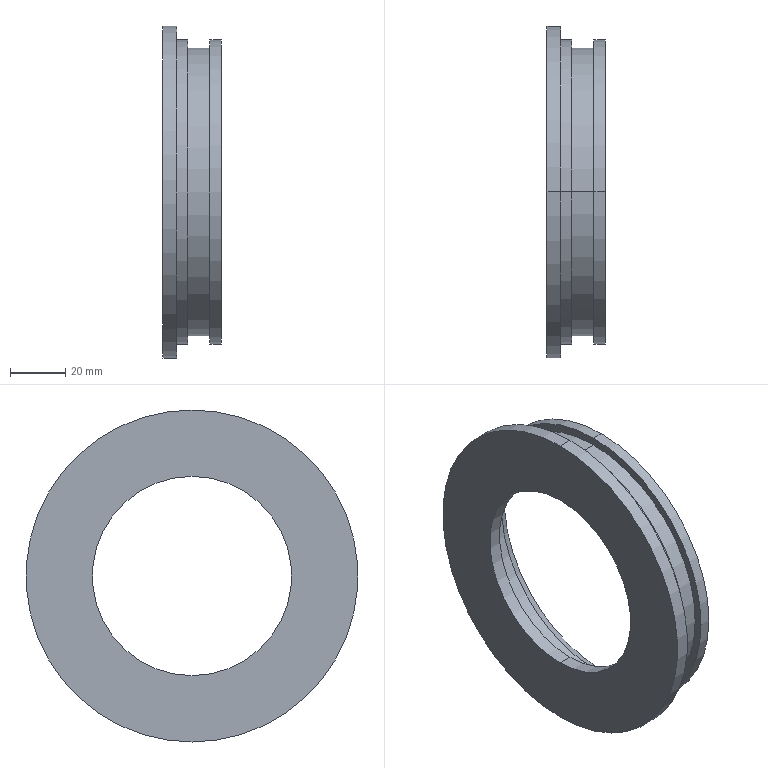Part | STEP file | AXIS_HOUSING_CLOSURE1V11 | 1 solid | 20 faces | box 21 x 120 x 120 mm | volume 65717 mm3 | cylinder 12 | plane 6 | cone 2 | commonest cylinder face diameters 110 x4 72 x2 95 x2 104 x2 120 x2
STEP:
#1=CARTESIAN_POINT('',(0.,0.,0.));
#2=DIRECTION('',(0.,0.,1.));
#3=DIRECTION('',(1.,0.,0.));
#4=AXIS2_PLACEMENT_3D('',#1,#2,#3);
#5=CARTESIAN_POINT('',(57.365,-30.,-47.5));
#6=VERTEX_POINT('',#5);
#7=CARTESIAN_POINT('',(60.829,-30.,-49.5));
#8=VERTEX_POINT('',#7);
#9=CARTESIAN_POINT('',(57.365,-30.,-47.5));
#10=DIRECTION('',(0.866,0.,-0.5));
#11=VECTOR('',#10,1.);
#12=LINE('',#9,#11);
#13=CARTESIAN_POINT('',(57.365,-30.,0.));
#14=DIRECTION('',(1.,0.,0.));
#15=DIRECTION('',(0.,0.,-1.));
#16=AXIS2_PLACEMENT_3D('',#13,#14,#15);
#17=CONICAL_SURFACE('',#16,47.5,0.5236);
#18=CARTESIAN_POINT('',(6.283,0.));
#19=DIRECTION('',(0.,1.));
#20=VECTOR('',#19,1.);
#21=LINE('',#18,#20);
#22=(GEOMETRIC_REPRESENTATION_CONTEXT(2)PARAMETRIC_REPRESENTATION_CONTEXT()REPRESENTATION_CONTEXT('',''));
#23=DEFINITIONAL_REPRESENTATION('',(#21),#22);
#24=PCURVE('',#17,#23);
#25=CARTESIAN_POINT('',(57.365,-30.,0.));
#26=DIRECTION('',(1.,0.,0.));
#27=DIRECTION('',(0.,0.,-1.));
#28=AXIS2_PLACEMENT_3D('',#25,#26,#27);
#29=CONICAL_SURFACE('',#28,47.5,0.5236);
#30=CARTESIAN_POINT('',(0.,0.));
#31=DIRECTION('',(0.,1.));
#32=VECTOR('',#31,1.);
#33=LINE('',#30,#32);
#34=(GEOMETRIC_REPRESENTATION_CONTEXT(2)PARAMETRIC_REPRESENTATION_CONTEXT()REPRESENTATION_CONTEXT('',''));
#35=DEFINITIONAL_REPRESENTATION('',(#33),#34);
#36=PCURVE('',#29,#35);
#37=SURFACE_CURVE('',#12,(#24,#36),.PCURVE_S1.);
#38=EDGE_CURVE('',#6,#8,#37,.T.);
#39=ORIENTED_EDGE('',*,*,#38,.T.);
#40=CARTESIAN_POINT('',(60.829,-30.,49.5));
#41=VERTEX_POINT('',#40);
#42=CARTESIAN_POINT('',(60.829,-30.,0.));
#43=DIRECTION('',(1.,0.,0.));
#44=DIRECTION('',(0.,0.,-1.));
#45=AXIS2_PLACEMENT_3D('',#42,#43,#44);
#46=CIRCLE('',#45,49.5);
#47=CARTESIAN_POINT('',(0.,3.464));
#48=DIRECTION('',(1.,0.));
#49=VECTOR('',#48,1.);
#50=LINE('',#47,#49);
#51=(GEOMETRIC_REPRESENTATION_CONTEXT(2)PARAMETRIC_REPRESENTATION_CONTEXT()REPRESENTATION_CONTEXT('',''));
#52=DEFINITIONAL_REPRESENTATION('',(#50),#51);
#53=PCURVE('',#17,#52);
#54=CARTESIAN_POINT('',(60.829,19.5,0.));
#55=DIRECTION('',(1.,0.,0.));
#56=DIRECTION('',(0.,0.,-1.));
#57=AXIS2_PLACEMENT_3D('',#54,#55,#56);
#58=PLANE('',#57);
#59=CARTESIAN_POINT('',(0.,-49.5));
#60=DIRECTION('',(1.,0.));
#61=AXIS2_PLACEMENT_2D('',#59,#60);
#62=CIRCLE('',#61,49.5);
#63=(GEOMETRIC_REPRESENTATION_CONTEXT(2)PARAMETRIC_REPRESENTATION_CONTEXT()REPRESENTATION_CONTEXT('',''));
#64=DEFINITIONAL_REPRESENTATION('',(#62),#63);
#65=PCURVE('',#58,#64);
#66=SURFACE_CURVE('',#46,(#53,#65),.PCURVE_S1.);
#67=EDGE_CURVE('',#41,#8,#66,.T.);
#68=ORIENTED_EDGE('',*,*,#67,.F.);
#69=CARTESIAN_POINT('',(57.365,-30.,47.5));
#70=VERTEX_POINT('',#69);
#71=CARTESIAN_POINT('',(57.365,-30.,47.5));
#72=DIRECTION('',(0.866,0.,0.5));
#73=VECTOR('',#72,1.);
#74=LINE('',#71,#73);
#75=CARTESIAN_POINT('',(3.142,0.));
#76=DIRECTION('',(0.,1.));
#77=VECTOR('',#76,1.);
#78=LINE('',#75,#77);
#79=(GEOMETRIC_REPRESENTATION_CONTEXT(2)PARAMETRIC_REPRESENTATION_CONTEXT()REPRESENTATION_CONTEXT('',''));
#80=DEFINITIONAL_REPRESENTATION('',(#78),#79);
#81=PCURVE('',#17,#80);
#82=CARTESIAN_POINT('',(3.142,0.));
#83=DIRECTION('',(0.,1.));
#84=VECTOR('',#83,1.);
#85=LINE('',#82,#84);
#86=(GEOMETRIC_REPRESENTATION_CONTEXT(2)PARAMETRIC_REPRESENTATION_CONTEXT()REPRESENTATION_CONTEXT('',''));
#87=DEFINITIONAL_REPRESENTATION('',(#85),#86);
#88=PCURVE('',#29,#87);
#89=SURFACE_CURVE('',#74,(#81,#88),.PCURVE_S1.);
#90=EDGE_CURVE('',#70,#41,#89,.T.);
#91=ORIENTED_EDGE('',*,*,#90,.F.);
#92=CARTESIAN_POINT('',(57.365,-30.,0.));
#93=DIRECTION('',(1.,0.,0.));
#94=DIRECTION('',(0.,0.,-1.));
#95=AXIS2_PLACEMENT_3D('',#92,#93,#94);
#96=CIRCLE('',#95,47.5);
#97=CARTESIAN_POINT('',(0.,0.));
#98=DIRECTION('',(1.,0.));
#99=VECTOR('',#98,1.);
#100=LINE('',#97,#99);
#101=(GEOMETRIC_REPRESENTATION_CONTEXT(2)PARAMETRIC_REPRESENTATION_CONTEXT()REPRESENTATION_CONTEXT('',''));
#102=DEFINITIONAL_REPRESENTATION('',(#100),#101);
#103=PCURVE('',#17,#102);
#104=CARTESIAN_POINT('',(39.829,-30.,0.));
#105=DIRECTION('',(1.,0.,0.));
#106=DIRECTION('',(0.,0.,-1.));
#107=AXIS2_PLACEMENT_3D('',#104,#105,#106);
#108=CYLINDRICAL_SURFACE('',#107,47.5);
#109=CARTESIAN_POINT('',(0.,17.536));
#110=DIRECTION('',(1.,0.));
#111=VECTOR('',#110,1.);
#112=LINE('',#109,#111);
#113=(GEOMETRIC_REPRESENTATION_CONTEXT(2)PARAMETRIC_REPRESENTATION_CONTEXT()REPRESENTATION_CONTEXT('',''));
#114=DEFINITIONAL_REPRESENTATION('',(#112),#113);
#115=PCURVE('',#108,#114);
#116=SURFACE_CURVE('',#96,(#103,#115),.PCURVE_S1.);
#117=EDGE_CURVE('',#70,#6,#116,.T.);
#118=ORIENTED_EDGE('',*,*,#117,.T.);
#119=EDGE_LOOP('',(#39,#68,#91,#118));
#120=FACE_BOUND('',#119,.F.);
#121=ADVANCED_FACE('',(#120),#17,.F.);
#122=CARTESIAN_POINT('',(44.829,-30.,-47.5));
#123=VERTEX_POINT('',#122);
#124=CARTESIAN_POINT('',(39.829,-30.,-47.5));
#125=DIRECTION('',(1.,0.,0.));
#126=VECTOR('',#125,1.);
#127=LINE('',#124,#126);
#128=CARTESIAN_POINT('',(6.283,0.));
#129=DIRECTION('',(0.,1.));
#130=VECTOR('',#129,1.);
#131=LINE('',#128,#130);
#132=(GEOMETRIC_REPRESENTATION_CONTEXT(2)PARAMETRIC_REPRESENTATION_CONTEXT()REPRESENTATION_CONTEXT('',''));
#133=DEFINITIONAL_REPRESENTATION('',(#131),#132);
#134=PCURVE('',#108,#133);
#135=CARTESIAN_POINT('',(39.829,-30.,0.));
#136=DIRECTION('',(1.,0.,0.));
#137=DIRECTION('',(0.,0.,-1.));
#138=AXIS2_PLACEMENT_3D('',#135,#136,#137);
#139=CYLINDRICAL_SURFACE('',#138,47.5);
#140=CARTESIAN_POINT('',(0.,0.));
#141=DIRECTION('',(0.,1.));
#142=VECTOR('',#141,1.);
#143=LINE('',#140,#142);
#144=(GEOMETRIC_REPRESENTATION_CONTEXT(2)PARAMETRIC_REPRESENTATION_CONTEXT()REPRESENTATION_CONTEXT('',''));
#145=DEFINITIONAL_REPRESENTATION('',(#143),#144);
#146=PCURVE('',#139,#145);
#147=SURFACE_CURVE('',#127,(#134,#146),.PCURVE_S1.);
#148=EDGE_CURVE('',#123,#6,#147,.T.);
#149=ORIENTED_EDGE('',*,*,#148,.T.);
#150=ORIENTED_EDGE('',*,*,#117,.F.);
#151=CARTESIAN_POINT('',(44.829,-30.,47.5));
#152=VERTEX_POINT('',#151);
#153=CARTESIAN_POINT('',(39.829,-30.,47.5));
#154=DIRECTION('',(1.,0.,0.));
#155=VECTOR('',#154,1.);
#156=LINE('',#153,#155);
#157=CARTESIAN_POINT('',(3.142,0.));
#158=DIRECTION('',(0.,1.));
#159=VECTOR('',#158,1.);
#160=LINE('',#157,#159);
#161=(GEOMETRIC_REPRESENTATION_CONTEXT(2)PARAMETRIC_REPRESENTATION_CONTEXT()REPRESENTATION_CONTEXT('',''));
#162=DEFINITIONAL_REPRESENTATION('',(#160),#161);
#163=PCURVE('',#108,#162);
#164=CARTESIAN_POINT('',(3.142,0.));
#165=DIRECTION('',(0.,1.));
#166=VECTOR('',#165,1.);
#167=LINE('',#164,#166);
#168=(GEOMETRIC_REPRESENTATION_CONTEXT(2)PARAMETRIC_REPRESENTATION_CONTEXT()REPRESENTATION_CONTEXT('',''));
#169=DEFINITIONAL_REPRESENTATION('',(#167),#168);
#170=PCURVE('',#139,#169);
#171=SURFACE_CURVE('',#156,(#163,#170),.PCURVE_S1.);
#172=EDGE_CURVE('',#152,#70,#171,.T.);
#173=ORIENTED_EDGE('',*,*,#172,.F.);
#174=CARTESIAN_POINT('',(44.829,-30.,0.));
#175=DIRECTION('',(1.,0.,0.));
#176=DIRECTION('',(0.,0.,-1.));
#177=AXIS2_PLACEMENT_3D('',#174,#175,#176);
#178=CIRCLE('',#177,47.5);
#179=CARTESIAN_POINT('',(0.,5.));
#180=DIRECTION('',(1.,0.));
#181=VECTOR('',#180,1.);
#182=LINE('',#179,#181);
#183=(GEOMETRIC_REPRESENTATION_CONTEXT(2)PARAMETRIC_REPRESENTATION_CONTEXT()REPRESENTATION_CONTEXT('',''));
#184=DEFINITIONAL_REPRESENTATION('',(#182),#183);
#185=PCURVE('',#108,#184);
#186=CARTESIAN_POINT('',(44.829,6.,0.));
#187=DIRECTION('',(1.,0.,0.));
#188=DIRECTION('',(0.,0.,-1.));
#189=AXIS2_PLACEMENT_3D('',#186,#187,#188);
#190=PLANE('',#189);
#191=CARTESIAN_POINT('',(0.,-36.));
#192=DIRECTION('',(1.,0.));
#193=AXIS2_PLACEMENT_2D('',#191,#192);
#194=CIRCLE('',#193,47.5);
#195=(GEOMETRIC_REPRESENTATION_CONTEXT(2)PARAMETRIC_REPRESENTATION_CONTEXT()REPRESENTATION_CONTEXT('',''));
#196=DEFINITIONAL_REPRESENTATION('',(#194),#195);
#197=PCURVE('',#190,#196);
#198=SURFACE_CURVE('',#178,(#185,#197),.PCURVE_S1.);
#199=EDGE_CURVE('',#152,#123,#198,.T.);
#200=ORIENTED_EDGE('',*,*,#199,.T.);
#201=EDGE_LOOP('',(#149,#150,#173,#200));
#202=FACE_BOUND('',#201,.F.);
#203=ADVANCED_FACE('',(#202),#108,.F.);
#204=CARTESIAN_POINT('',(39.829,-30.,-36.));
#205=VERTEX_POINT('',#204);
#206=CARTESIAN_POINT('',(44.829,-30.,-36.));
#207=VERTEX_POINT('',#206);
#208=CARTESIAN_POINT('',(39.829,-30.,-36.));
#209=DIRECTION('',(1.,0.,0.));
#210=VECTOR('',#209,1.);
#211=LINE('',#208,#210);
#212=CARTESIAN_POINT('',(39.829,-30.,0.));
#213=DIRECTION('',(1.,0.,0.));
#214=DIRECTION('',(0.,0.,-1.));
#215=AXIS2_PLACEMENT_3D('',#212,#213,#214);
#216=CYLINDRICAL_SURFACE('',#215,36.);
#217=CARTESIAN_POINT('',(6.283,0.));
#218=DIRECTION('',(0.,1.));
#219=VECTOR('',#218,1.);
#220=LINE('',#217,#219);
#221=(GEOMETRIC_REPRESENTATION_CONTEXT(2)PARAMETRIC_REPRESENTATION_CONTEXT()REPRESENTATION_CONTEXT('',''));
#222=DEFINITIONAL_REPRESENTATION('',(#220),#221);
#223=PCURVE('',#216,#222);
#224=CARTESIAN_POINT('',(39.829,-30.,0.));
#225=DIRECTION('',(1.,0.,0.));
#226=DIRECTION('',(0.,0.,-1.));
#227=AXIS2_PLACEMENT_3D('',#224,#225,#226);
#228=CYLINDRICAL_SURFACE('',#227,36.);
#229=CARTESIAN_POINT('',(0.,0.));
#230=DIRECTION('',(0.,1.));
#231=VECTOR('',#230,1.);
#232=LINE('',#229,#231);
#233=(GEOMETRIC_REPRESENTATION_CONTEXT(2)PARAMETRIC_REPRESENTATION_CONTEXT()REPRESENTATION_CONTEXT('',''));
#234=DEFINITIONAL_REPRESENTATION('',(#232),#233);
#235=PCURVE('',#228,#234);
#236=SURFACE_CURVE('',#211,(#223,#235),.PCURVE_S1.);
#237=EDGE_CURVE('',#205,#207,#236,.T.);
#238=ORIENTED_EDGE('',*,*,#237,.T.);
#239=CARTESIAN_POINT('',(44.829,-30.,36.));
#240=VERTEX_POINT('',#239);
#241=CARTESIAN_POINT('',(44.829,-30.,0.));
#242=DIRECTION('',(1.,0.,0.));
#243=DIRECTION('',(0.,0.,-1.));
#244=AXIS2_PLACEMENT_3D('',#241,#242,#243);
#245=CIRCLE('',#244,36.);
#246=CARTESIAN_POINT('',(0.,5.));
#247=DIRECTION('',(1.,0.));
#248=VECTOR('',#247,1.);
#249=LINE('',#246,#248);
#250=(GEOMETRIC_REPRESENTATION_CONTEXT(2)PARAMETRIC_REPRESENTATION_CONTEXT()REPRESENTATION_CONTEXT('',''));
#251=DEFINITIONAL_REPRESENTATION('',(#249),#250);
#252=PCURVE('',#216,#251);
#253=CARTESIAN_POINT('',(0.,-36.));
#254=DIRECTION('',(1.,0.));
#255=AXIS2_PLACEMENT_2D('',#253,#254);
#256=CIRCLE('',#255,36.);
#257=(GEOMETRIC_REPRESENTATION_CONTEXT(2)PARAMETRIC_REPRESENTATION_CONTEXT()REPRESENTATION_CONTEXT('',''));
#258=DEFINITIONAL_REPRESENTATION('',(#256),#257);
#259=PCURVE('',#190,#258);
#260=SURFACE_CURVE('',#245,(#252,#259),.PCURVE_S1.);
#261=EDGE_CURVE('',#240,#207,#260,.T.);
#262=ORIENTED_EDGE('',*,*,#261,.F.);
#263=CARTESIAN_POINT('',(39.829,-30.,36.));
#264=VERTEX_POINT('',#263);
#265=CARTESIAN_POINT('',(39.829,-30.,36.));
#266=DIRECTION('',(1.,0.,0.));
#267=VECTOR('',#266,1.);
#268=LINE('',#265,#267);
#269=CARTESIAN_POINT('',(3.142,0.));
#270=DIRECTION('',(0.,1.));
#271=VECTOR('',#270,1.);
#272=LINE('',#269,#271);
#273=(GEOMETRIC_REPRESENTATION_CONTEXT(2)PARAMETRIC_REPRESENTATION_CONTEXT()REPRESENTATION_CONTEXT('',''));
#274=DEFINITIONAL_REPRESENTATION('',(#272),#273);
#275=PCURVE('',#216,#274);
#276=CARTESIAN_POINT('',(3.142,0.));
#277=DIRECTION('',(0.,1.));
#278=VECTOR('',#277,1.);
#279=LINE('',#276,#278);
#280=(GEOMETRIC_REPRESENTATION_CONTEXT(2)PARAMETRIC_REPRESENTATION_CONTEXT()REPRESENTATION_CONTEXT('',''));
#281=DEFINITIONAL_REPRESENTATION('',(#279),#280);
#282=PCURVE('',#228,#281);
#283=SURFACE_CURVE('',#268,(#275,#282),.PCURVE_S1.);
#284=EDGE_CURVE('',#264,#240,#283,.T.);
#285=ORIENTED_EDGE('',*,*,#284,.F.);
#286=CARTESIAN_POINT('',(39.829,-30.,0.));
#287=DIRECTION('',(1.,0.,0.));
#288=DIRECTION('',(0.,0.,-1.));
#289=AXIS2_PLACEMENT_3D('',#286,#287,#288);
#290=CIRCLE('',#289,36.);
#291=CARTESIAN_POINT('',(0.,0.));
#292=DIRECTION('',(1.,0.));
#293=VECTOR('',#292,1.);
#294=LINE('',#291,#293);
#295=(GEOMETRIC_REPRESENTATION_CONTEXT(2)PARAMETRIC_REPRESENTATION_CONTEXT()REPRESENTATION_CONTEXT('',''));
#296=DEFINITIONAL_REPRESENTATION('',(#294),#295);
#297=PCURVE('',#216,#296);
#298=CARTESIAN_POINT('',(39.829,30.,0.));
#299=DIRECTION('',(-1.,0.,0.));
#300=DIRECTION('',(0.,0.,1.));
#301=AXIS2_PLACEMENT_3D('',#298,#299,#300);
#302=PLANE('',#301);
#303=CARTESIAN_POINT('',(-36.,-60.));
#304=CARTESIAN_POINT('',(-36.,2.354));
#305=CARTESIAN_POINT('',(18.,-28.823));
#306=CARTESIAN_POINT('',(72.,-60.));
#307=CARTESIAN_POINT('',(18.,-91.177));
#308=CARTESIAN_POINT('',(-36.,-122.354));
#309=CARTESIAN_POINT('',(-36.,-60.));
#310=(BOUNDED_CURVE()B_SPLINE_CURVE(2,(#303,#304,#305,#306,#307,#308,#309),.UNSPECIFIED.,.T.,.F.)B_SPLINE_CURVE_WITH_KNOTS((1,2,2,2,2,1),(-2.094,0.,2.094,4.189,6.283,8.378),.UNSPECIFIED.)CURVE()GEOMETRIC_REPRESENTATION_ITEM()RATIONAL_B_SPLINE_CURVE((1.,0.5,1.,0.5,1.,0.5,1.))REPRESENTATION_ITEM(''));
#311=(GEOMETRIC_REPRESENTATION_CONTEXT(2)PARAMETRIC_REPRESENTATION_CONTEXT()REPRESENTATION_CONTEXT('',''));
#312=DEFINITIONAL_REPRESENTATION('',(#310),#311);
#313=PCURVE('',#302,#312);
#314=SURFACE_CURVE('',#290,(#297,#313),.PCURVE_S1.);
#315=EDGE_CURVE('',#264,#205,#314,.T.);
#316=ORIENTED_EDGE('',*,*,#315,.T.);
#317=EDGE_LOOP('',(#238,#262,#285,#316));
#318=FACE_BOUND('',#317,.F.);
#319=ADVANCED_FACE('',(#318),#216,.F.);
#320=CARTESIAN_POINT('',(39.829,-30.,-60.));
#321=VERTEX_POINT('',#320);
#322=CARTESIAN_POINT('',(39.829,-30.,60.));
#323=VERTEX_POINT('',#322);
#324=CARTESIAN_POINT('',(39.829,-30.,0.));
#325=DIRECTION('',(1.,0.,0.));
#326=DIRECTION('',(0.,0.,-1.));
#327=AXIS2_PLACEMENT_3D('',#324,#325,#326);
#328=CIRCLE('',#327,60.);
#329=CARTESIAN_POINT('',(39.829,-30.,0.));
#330=DIRECTION('',(1.,0.,0.));
#331=DIRECTION('',(0.,0.,-1.));
#332=AXIS2_PLACEMENT_3D('',#329,#330,#331);
#333=CYLINDRICAL_SURFACE('',#332,60.);
#334=CARTESIAN_POINT('',(0.,0.));
#335=DIRECTION('',(1.,0.));
#336=VECTOR('',#335,1.);
#337=LINE('',#334,#336);
#338=(GEOMETRIC_REPRESENTATION_CONTEXT(2)PARAMETRIC_REPRESENTATION_CONTEXT()REPRESENTATION_CONTEXT('',''));
#339=DEFINITIONAL_REPRESENTATION('',(#337),#338);
#340=PCURVE('',#333,#339);
#341=CARTESIAN_POINT('',(-60.,-60.));
#342=CARTESIAN_POINT('',(-60.,43.923));
#343=CARTESIAN_POINT('',(30.,-8.038));
#344=CARTESIAN_POINT('',(120.,-60.));
#345=CARTESIAN_POINT('',(30.,-111.962));
#346=CARTESIAN_POINT('',(-60.,-163.923));
#347=CARTESIAN_POINT('',(-60.,-60.));
#348=(BOUNDED_CURVE()B_SPLINE_CURVE(2,(#341,#342,#343,#344,#345,#346,#347),.UNSPECIFIED.,.T.,.F.)B_SPLINE_CURVE_WITH_KNOTS((1,2,2,2,2,1),(-2.094,0.,2.094,4.189,6.283,8.378),.UNSPECIFIED.)CURVE()GEOMETRIC_REPRESENTATION_ITEM()RATIONAL_B_SPLINE_CURVE((1.,0.5,1.,0.5,1.,0.5,1.))REPRESENTATION_ITEM(''));
#349=(GEOMETRIC_REPRESENTATION_CONTEXT(2)PARAMETRIC_REPRESENTATION_CONTEXT()REPRESENTATION_CONTEXT('',''));
#350=DEFINITIONAL_REPRESENTATION('',(#348),#349);
#351=PCURVE('',#302,#350);
#352=SURFACE_CURVE('',#328,(#340,#351),.PCURVE_S1.);
#353=EDGE_CURVE('',#321,#323,#352,.T.);
#354=ORIENTED_EDGE('',*,*,#353,.T.);
#355=CARTESIAN_POINT('',(44.829,-30.,60.));
#356=VERTEX_POINT('',#355);
#357=CARTESIAN_POINT('',(39.829,-30.,60.));
#358=DIRECTION('',(1.,0.,0.));
#359=VECTOR('',#358,1.);
#360=LINE('',#357,#359);
#361=CARTESIAN_POINT('',(3.142,0.));
#362=DIRECTION('',(0.,1.));
#363=VECTOR('',#362,1.);
#364=LINE('',#361,#363);
#365=(GEOMETRIC_REPRESENTATION_CONTEXT(2)PARAMETRIC_REPRESENTATION_CONTEXT()REPRESENTATION_CONTEXT('',''));
#366=DEFINITIONAL_REPRESENTATION('',(#364),#365);
#367=PCURVE('',#333,#366);
#368=CARTESIAN_POINT('',(39.829,-30.,0.));
#369=DIRECTION('',(1.,0.,0.));
#370=DIRECTION('',(0.,0.,-1.));
#371=AXIS2_PLACEMENT_3D('',#368,#369,#370);
#372=CYLINDRICAL_SURFACE('',#371,60.);
#373=CARTESIAN_POINT('',(3.142,0.));
#374=DIRECTION('',(0.,1.));
#375=VECTOR('',#374,1.);
#376=LINE('',#373,#375);
#377=(GEOMETRIC_REPRESENTATION_CONTEXT(2)PARAMETRIC_REPRESENTATION_CONTEXT()REPRESENTATION_CONTEXT('',''));
#378=DEFINITIONAL_REPRESENTATION('',(#376),#377);
#379=PCURVE('',#372,#378);
#380=SURFACE_CURVE('',#360,(#367,#379),.PCURVE_S1.);
#381=EDGE_CURVE('',#323,#356,#380,.T.);
#382=ORIENTED_EDGE('',*,*,#381,.T.);
#383=CARTESIAN_POINT('',(44.829,-30.,-60.));
#384=VERTEX_POINT('',#383);
#385=CARTESIAN_POINT('',(44.829,-30.,0.));
#386=DIRECTION('',(1.,0.,0.));
#387=DIRECTION('',(0.,0.,-1.));
#388=AXIS2_PLACEMENT_3D('',#385,#386,#387);
#389=CIRCLE('',#388,60.);
#390=CARTESIAN_POINT('',(0.,5.));
#391=DIRECTION('',(1.,0.));
#392=VECTOR('',#391,1.);
#393=LINE('',#390,#392);
#394=(GEOMETRIC_REPRESENTATION_CONTEXT(2)PARAMETRIC_REPRESENTATION_CONTEXT()REPRESENTATION_CONTEXT('',''));
#395=DEFINITIONAL_REPRESENTATION('',(#393),#394);
#396=PCURVE('',#333,#395);
#397=CARTESIAN_POINT('',(44.829,25.,0.));
#398=DIRECTION('',(1.,0.,0.));
#399=DIRECTION('',(0.,0.,-1.));
#400=AXIS2_PLACEMENT_3D('',#397,#398,#399);
#401=PLANE('',#400);
#402=CARTESIAN_POINT('',(0.,-55.));
#403=DIRECTION('',(1.,0.));
#404=AXIS2_PLACEMENT_2D('',#402,#403);
#405=CIRCLE('',#404,60.);
#406=(GEOMETRIC_REPRESENTATION_CONTEXT(2)PARAMETRIC_REPRESENTATION_CONTEXT()REPRESENTATION_CONTEXT('',''));
#407=DEFINITIONAL_REPRESENTATION('',(#405),#406);
#408=PCURVE('',#401,#407);
#409=SURFACE_CURVE('',#389,(#396,#408),.PCURVE_S1.);
#410=EDGE_CURVE('',#384,#356,#409,.T.);
#411=ORIENTED_EDGE('',*,*,#410,.F.);
#412=CARTESIAN_POINT('',(39.829,-30.,-60.));
#413=DIRECTION('',(1.,0.,0.));
#414=VECTOR('',#413,1.);
#415=LINE('',#412,#414);
#416=CARTESIAN_POINT('',(0.,0.));
#417=DIRECTION('',(0.,1.));
#418=VECTOR('',#417,1.);
#419=LINE('',#416,#418);
#420=(GEOMETRIC_REPRESENTATION_CONTEXT(2)PARAMETRIC_REPRESENTATION_CONTEXT()REPRESENTATION_CONTEXT('',''));
#421=DEFINITIONAL_REPRESENTATION('',(#419),#420);
#422=PCURVE('',#333,#421);
#423=CARTESIAN_POINT('',(6.283,0.));
#424=DIRECTION('',(0.,1.));
#425=VECTOR('',#424,1.);
#426=LINE('',#423,#425);
#427=(GEOMETRIC_REPRESENTATION_CONTEXT(2)PARAMETRIC_REPRESENTATION_CONTEXT()REPRESENTATION_CONTEXT('',''));
#428=DEFINITIONAL_REPRESENTATION('',(#426),#427);
#429=PCURVE('',#372,#428);
#430=SURFACE_CURVE('',#415,(#422,#429),.PCURVE_S1.);
#431=EDGE_CURVE('',#321,#384,#430,.T.);
#432=ORIENTED_EDGE('',*,*,#431,.F.);
#433=EDGE_LOOP('',(#354,#382,#411,#432));
#434=FACE_BOUND('',#433,.T.);
#435=ADVANCED_FACE('',(#434),#333,.T.);
#436=CARTESIAN_POINT('',(44.829,-30.,-55.));
#437=VERTEX_POINT('',#436);
#438=CARTESIAN_POINT('',(44.829,-30.,55.));
#439=VERTEX_POINT('',#438);
#440=CARTESIAN_POINT('',(44.829,-30.,0.));
#441=DIRECTION('',(1.,0.,0.));
#442=DIRECTION('',(0.,0.,-1.));
#443=AXIS2_PLACEMENT_3D('',#440,#441,#442);
#444=CIRCLE('',#443,55.);
#445=CARTESIAN_POINT('',(39.829,-30.,0.));
#446=DIRECTION('',(1.,0.,0.));
#447=DIRECTION('',(0.,0.,-1.));
#448=AXIS2_PLACEMENT_3D('',#445,#446,#447);
#449=CYLINDRICAL_SURFACE('',#448,55.);
#450=CARTESIAN_POINT('',(0.,5.));
#451=DIRECTION('',(1.,0.));
#452=VECTOR('',#451,1.);
#453=LINE('',#450,#452);
#454=(GEOMETRIC_REPRESENTATION_CONTEXT(2)PARAMETRIC_REPRESENTATION_CONTEXT()REPRESENTATION_CONTEXT('',''));
#455=DEFINITIONAL_REPRESENTATION('',(#453),#454);
#456=PCURVE('',#449,#455);
#457=CARTESIAN_POINT('',(0.,-55.));
#458=DIRECTION('',(1.,0.));
#459=AXIS2_PLACEMENT_2D('',#457,#458);
#460=CIRCLE('',#459,55.);
#461=(GEOMETRIC_REPRESENTATION_CONTEXT(2)PARAMETRIC_REPRESENTATION_CONTEXT()REPRESENTATION_CONTEXT('',''));
#462=DEFINITIONAL_REPRESENTATION('',(#460),#461);
#463=PCURVE('',#401,#462);
#464=SURFACE_CURVE('',#444,(#456,#463),.PCURVE_S1.);
#465=EDGE_CURVE('',#437,#439,#464,.T.);
#466=ORIENTED_EDGE('',*,*,#465,.T.);
#467=CARTESIAN_POINT('',(48.829,-30.,55.));
#468=VERTEX_POINT('',#467);
#469=CARTESIAN_POINT('',(39.829,-30.,55.));
#470=DIRECTION('',(1.,0.,0.));
#471=VECTOR('',#470,1.);
#472=LINE('',#469,#471);
#473=CARTESIAN_POINT('',(3.142,0.));
#474=DIRECTION('',(0.,1.));
#475=VECTOR('',#474,1.);
#476=LINE('',#473,#475);
#477=(GEOMETRIC_REPRESENTATION_CONTEXT(2)PARAMETRIC_REPRESENTATION_CONTEXT()REPRESENTATION_CONTEXT('',''));
#478=DEFINITIONAL_REPRESENTATION('',(#476),#477);
#479=PCURVE('',#449,#478);
#480=CARTESIAN_POINT('',(39.829,-30.,0.));
#481=DIRECTION('',(1.,0.,0.));
#482=DIRECTION('',(0.,0.,-1.));
#483=AXIS2_PLACEMENT_3D('',#480,#481,#482);
#484=CYLINDRICAL_SURFACE('',#483,55.);
#485=CARTESIAN_POINT('',(3.142,0.));
#486=DIRECTION('',(0.,1.));
#487=VECTOR('',#486,1.);
#488=LINE('',#485,#487);
#489=(GEOMETRIC_REPRESENTATION_CONTEXT(2)PARAMETRIC_REPRESENTATION_CONTEXT()REPRESENTATION_CONTEXT('',''));
#490=DEFINITIONAL_REPRESENTATION('',(#488),#489);
#491=PCURVE('',#484,#490);
#492=SURFACE_CURVE('',#472,(#479,#491),.PCURVE_S1.);
#493=EDGE_CURVE('',#439,#468,#492,.T.);
#494=ORIENTED_EDGE('',*,*,#493,.T.);
#495=CARTESIAN_POINT('',(48.829,-30.,-55.));
#496=VERTEX_POINT('',#495);
#497=CARTESIAN_POINT('',(48.829,-30.,0.));
#498=DIRECTION('',(1.,0.,0.));
#499=DIRECTION('',(0.,0.,-1.));
#500=AXIS2_PLACEMENT_3D('',#497,#498,#499);
#501=CIRCLE('',#500,55.);
#502=CARTESIAN_POINT('',(0.,9.));
#503=DIRECTION('',(1.,0.));
#504=VECTOR('',#503,1.);
#505=LINE('',#502,#504);
#506=(GEOMETRIC_REPRESENTATION_CONTEXT(2)PARAMETRIC_REPRESENTATION_CONTEXT()REPRESENTATION_CONTEXT('',''));
#507=DEFINITIONAL_REPRESENTATION('',(#505),#506);
#508=PCURVE('',#449,#507);
#509=CARTESIAN_POINT('',(48.829,22.,0.));
#510=DIRECTION('',(1.,0.,0.));
#511=DIRECTION('',(0.,0.,-1.));
#512=AXIS2_PLACEMENT_3D('',#509,#510,#511);
#513=PLANE('',#512);
#514=CARTESIAN_POINT('',(0.,-52.));
#515=DIRECTION('',(1.,0.));
#516=AXIS2_PLACEMENT_2D('',#514,#515);
#517=CIRCLE('',#516,55.);
#518=(GEOMETRIC_REPRESENTATION_CONTEXT(2)PARAMETRIC_REPRESENTATION_CONTEXT()REPRESENTATION_CONTEXT('',''));
#519=DEFINITIONAL_REPRESENTATION('',(#517),#518);
#520=PCURVE('',#513,#519);
#521=SURFACE_CURVE('',#501,(#508,#520),.PCURVE_S1.);
#522=EDGE_CURVE('',#496,#468,#521,.T.);
#523=ORIENTED_EDGE('',*,*,#522,.F.);
#524=CARTESIAN_POINT('',(39.829,-30.,-55.));
#525=DIRECTION('',(1.,0.,0.));
#526=VECTOR('',#525,1.);
#527=LINE('',#524,#526);
#528=CARTESIAN_POINT('',(0.,0.));
#529=DIRECTION('',(0.,1.));
#530=VECTOR('',#529,1.);
#531=LINE('',#528,#530);
#532=(GEOMETRIC_REPRESENTATION_CONTEXT(2)PARAMETRIC_REPRESENTATION_CONTEXT()REPRESENTATION_CONTEXT('',''));
#533=DEFINITIONAL_REPRESENTATION('',(#531),#532);
#534=PCURVE('',#449,#533);
#535=CARTESIAN_POINT('',(6.283,0.));
#536=DIRECTION('',(0.,1.));
#537=VECTOR('',#536,1.);
#538=LINE('',#535,#537);
#539=(GEOMETRIC_REPRESENTATION_CONTEXT(2)PARAMETRIC_REPRESENTATION_CONTEXT()REPRESENTATION_CONTEXT('',''));
#540=DEFINITIONAL_REPRESENTATION('',(#538),#539);
#541=PCURVE('',#484,#540);
#542=SURFACE_CURVE('',#527,(#534,#541),.PCURVE_S1.);
#543=EDGE_CURVE('',#437,#496,#542,.T.);
#544=ORIENTED_EDGE('',*,*,#543,.F.);
#545=EDGE_LOOP('',(#466,#494,#523,#544));
#546=FACE_BOUND('',#545,.T.);
#547=ADVANCED_FACE('',(#546),#449,.T.);
#548=CARTESIAN_POINT('',(48.829,-30.,-52.));
#549=VERTEX_POINT('',#548);
#550=CARTESIAN_POINT('',(48.829,-30.,52.));
#551=VERTEX_POINT('',#550);
#552=CARTESIAN_POINT('',(48.829,-30.,0.));
#553=DIRECTION('',(1.,0.,0.));
#554=DIRECTION('',(0.,0.,-1.));
#555=AXIS2_PLACEMENT_3D('',#552,#553,#554);
#556=CIRCLE('',#555,52.);
#557=CARTESIAN_POINT('',(39.829,-30.,0.));
#558=DIRECTION('',(1.,0.,0.));
#559=DIRECTION('',(0.,0.,-1.));
#560=AXIS2_PLACEMENT_3D('',#557,#558,#559);
#561=CYLINDRICAL_SURFACE('',#560,52.);
#562=CARTESIAN_POINT('',(0.,9.));
#563=DIRECTION('',(1.,0.));
#564=VECTOR('',#563,1.);
#565=LINE('',#562,#564);
#566=(GEOMETRIC_REPRESENTATION_CONTEXT(2)PARAMETRIC_REPRESENTATION_CONTEXT()REPRESENTATION_CONTEXT('',''));
#567=DEFINITIONAL_REPRESENTATION('',(#565),#566);
#568=PCURVE('',#561,#567);
#569=CARTESIAN_POINT('',(0.,-52.));
#570=DIRECTION('',(1.,0.));
#571=AXIS2_PLACEMENT_2D('',#569,#570);
#572=CIRCLE('',#571,52.);
#573=(GEOMETRIC_REPRESENTATION_CONTEXT(2)PARAMETRIC_REPRESENTATION_CONTEXT()REPRESENTATION_CONTEXT('',''));
#574=DEFINITIONAL_REPRESENTATION('',(#572),#573);
#575=PCURVE('',#513,#574);
#576=SURFACE_CURVE('',#556,(#568,#575),.PCURVE_S1.);
#577=EDGE_CURVE('',#549,#551,#576,.T.);
#578=ORIENTED_EDGE('',*,*,#577,.T.);
#579=CARTESIAN_POINT('',(56.829,-30.,52.));
#580=VERTEX_POINT('',#579);
#581=CARTESIAN_POINT('',(39.829,-30.,52.));
#582=DIRECTION('',(1.,0.,0.));
#583=VECTOR('',#582,1.);
#584=LINE('',#581,#583);
#585=CARTESIAN_POINT('',(3.142,0.));
#586=DIRECTION('',(0.,1.));
#587=VECTOR('',#586,1.);
#588=LINE('',#585,#587);
#589=(GEOMETRIC_REPRESENTATION_CONTEXT(2)PARAMETRIC_REPRESENTATION_CONTEXT()REPRESENTATION_CONTEXT('',''));
#590=DEFINITIONAL_REPRESENTATION('',(#588),#589);
#591=PCURVE('',#561,#590);
#592=CARTESIAN_POINT('',(39.829,-30.,0.));
#593=DIRECTION('',(1.,0.,0.));
#594=DIRECTION('',(0.,0.,-1.));
#595=AXIS2_PLACEMENT_3D('',#592,#593,#594);
#596=CYLINDRICAL_SURFACE('',#595,52.);
#597=CARTESIAN_POINT('',(3.142,0.));
#598=DIRECTION('',(0.,1.));
#599=VECTOR('',#598,1.);
#600=LINE('',#597,#599);
#601=(GEOMETRIC_REPRESENTATION_CONTEXT(2)PARAMETRIC_REPRESENTATION_CONTEXT()REPRESENTATION_CONTEXT('',''));
#602=DEFINITIONAL_REPRESENTATION('',(#600),#601);
#603=PCURVE('',#596,#602);
#604=SURFACE_CURVE('',#584,(#591,#603),.PCURVE_S1.);
#605=EDGE_CURVE('',#551,#580,#604,.T.);
#606=ORIENTED_EDGE('',*,*,#605,.T.);
#607=CARTESIAN_POINT('',(56.829,-30.,-52.));
#608=VERTEX_POINT('',#607);
#609=CARTESIAN_POINT('',(56.829,-30.,0.));
#610=DIRECTION('',(1.,0.,0.));
#611=DIRECTION('',(0.,0.,-1.));
#612=AXIS2_PLACEMENT_3D('',#609,#610,#611);
#613=CIRCLE('',#612,52.);
#614=CARTESIAN_POINT('',(0.,17.));
#615=DIRECTION('',(1.,0.));
#616=VECTOR('',#615,1.);
#617=LINE('',#614,#616);
#618=(GEOMETRIC_REPRESENTATION_CONTEXT(2)PARAMETRIC_REPRESENTATION_CONTEXT()REPRESENTATION_CONTEXT('',''));
#619=DEFINITIONAL_REPRESENTATION('',(#617),#618);
#620=PCURVE('',#561,#619);
#621=CARTESIAN_POINT('',(56.829,25.,0.));
#622=DIRECTION('',(-1.,0.,0.));
#623=DIRECTION('',(0.,0.,1.));
#624=AXIS2_PLACEMENT_3D('',#621,#622,#623);
#625=PLANE('',#624);
#626=CARTESIAN_POINT('',(-52.,-55.));
#627=CARTESIAN_POINT('',(-52.,35.067));
#628=CARTESIAN_POINT('',(26.,-9.967));
#629=CARTESIAN_POINT('',(104.,-55.));
#630=CARTESIAN_POINT('',(26.,-100.033));
#631=CARTESIAN_POINT('',(-52.,-145.067));
#632=CARTESIAN_POINT('',(-52.,-55.));
#633=(BOUNDED_CURVE()B_SPLINE_CURVE(2,(#626,#627,#628,#629,#630,#631,#632),.UNSPECIFIED.,.T.,.F.)B_SPLINE_CURVE_WITH_KNOTS((1,2,2,2,2,1),(-2.094,0.,2.094,4.189,6.283,8.378),.UNSPECIFIED.)CURVE()GEOMETRIC_REPRESENTATION_ITEM()RATIONAL_B_SPLINE_CURVE((1.,0.5,1.,0.5,1.,0.5,1.))REPRESENTATION_ITEM(''));
#634=(GEOMETRIC_REPRESENTATION_CONTEXT(2)PARAMETRIC_REPRESENTATION_CONTEXT()REPRESENTATION_CONTEXT('',''));
#635=DEFINITIONAL_REPRESENTATION('',(#633),#634);
#636=PCURVE('',#625,#635);
#637=SURFACE_CURVE('',#613,(#620,#636),.PCURVE_S1.);
#638=EDGE_CURVE('',#608,#580,#637,.T.);
#639=ORIENTED_EDGE('',*,*,#638,.F.);
#640=CARTESIAN_POINT('',(39.829,-30.,-52.));
#641=DIRECTION('',(1.,0.,0.));
#642=VECTOR('',#641,1.);
#643=LINE('',#640,#642);
#644=CARTESIAN_POINT('',(0.,0.));
#645=DIRECTION('',(0.,1.));
#646=VECTOR('',#645,1.);
#647=LINE('',#644,#646);
#648=(GEOMETRIC_REPRESENTATION_CONTEXT(2)PARAMETRIC_REPRESENTATION_CONTEXT()REPRESENTATION_CONTEXT('',''));
#649=DEFINITIONAL_REPRESENTATION('',(#647),#648);
#650=PCURVE('',#561,#649);
#651=CARTESIAN_POINT('',(6.283,0.));
#652=DIRECTION('',(0.,1.));
#653=VECTOR('',#652,1.);
#654=LINE('',#651,#653);
#655=(GEOMETRIC_REPRESENTATION_CONTEXT(2)PARAMETRIC_REPRESENTATION_CONTEXT()REPRESENTATION_CONTEXT('',''));
#656=DEFINITIONAL_REPRESENTATION('',(#654),#655);
#657=PCURVE('',#596,#656);
#658=SURFACE_CURVE('',#643,(#650,#657),.PCURVE_S1.);
#659=EDGE_CURVE('',#549,#608,#658,.T.);
#660=ORIENTED_EDGE('',*,*,#659,.F.);
#661=EDGE_LOOP('',(#578,#606,#639,#660));
#662=FACE_BOUND('',#661,.T.);
#663=ADVANCED_FACE('',(#662),#561,.T.);
#664=CARTESIAN_POINT('',(56.829,-30.,-55.));
#665=VERTEX_POINT('',#664);
#666=CARTESIAN_POINT('',(56.829,-30.,55.));
#667=VERTEX_POINT('',#666);
#668=CARTESIAN_POINT('',(56.829,-30.,0.));
#669=DIRECTION('',(1.,0.,0.));
#670=DIRECTION('',(0.,0.,-1.));
#671=AXIS2_PLACEMENT_3D('',#668,#669,#670);
#672=CIRCLE('',#671,55.);
#673=CARTESIAN_POINT('',(39.829,-30.,0.));
#674=DIRECTION('',(1.,0.,0.));
#675=DIRECTION('',(0.,0.,-1.));
#676=AXIS2_PLACEMENT_3D('',#673,#674,#675);
#677=CYLINDRICAL_SURFACE('',#676,55.);
#678=CARTESIAN_POINT('',(0.,17.));
#679=DIRECTION('',(1.,0.));
#680=VECTOR('',#679,1.);
#681=LINE('',#678,#680);
#682=(GEOMETRIC_REPRESENTATION_CONTEXT(2)PARAMETRIC_REPRESENTATION_CONTEXT()REPRESENTATION_CONTEXT('',''));
#683=DEFINITIONAL_REPRESENTATION('',(#681),#682);
#684=PCURVE('',#677,#683);
#685=CARTESIAN_POINT('',(-55.,-55.));
#686=CARTESIAN_POINT('',(-55.,40.263));
#687=CARTESIAN_POINT('',(27.5,-7.369));
#688=CARTESIAN_POINT('',(110.,-55.));
#689=CARTESIAN_POINT('',(27.5,-102.631));
#690=CARTESIAN_POINT('',(-55.,-150.263));
#691=CARTESIAN_POINT('',(-55.,-55.));
#692=(BOUNDED_CURVE()B_SPLINE_CURVE(2,(#685,#686,#687,#688,#689,#690,#691),.UNSPECIFIED.,.T.,.F.)B_SPLINE_CURVE_WITH_KNOTS((1,2,2,2,2,1),(-2.094,0.,2.094,4.189,6.283,8.378),.UNSPECIFIED.)CURVE()GEOMETRIC_REPRESENTATION_ITEM()RATIONAL_B_SPLINE_CURVE((1.,0.5,1.,0.5,1.,0.5,1.))REPRESENTATION_ITEM(''));
#693=(GEOMETRIC_REPRESENTATION_CONTEXT(2)PARAMETRIC_REPRESENTATION_CONTEXT()REPRESENTATION_CONTEXT('',''));
#694=DEFINITIONAL_REPRESENTATION('',(#692),#693);
#695=PCURVE('',#625,#694);
#696=SURFACE_CURVE('',#672,(#684,#695),.PCURVE_S1.);
#697=EDGE_CURVE('',#665,#667,#696,.T.);
#698=ORIENTED_EDGE('',*,*,#697,.T.);
#699=CARTESIAN_POINT('',(60.829,-30.,55.));
#700=VERTEX_POINT('',#699);
#701=CARTESIAN_POINT('',(39.829,-30.,55.));
#702=DIRECTION('',(1.,0.,0.));
#703=VECTOR('',#702,1.);
#704=LINE('',#701,#703);
#705=CARTESIAN_POINT('',(3.142,0.));
#706=DIRECTION('',(0.,1.));
#707=VECTOR('',#706,1.);
#708=LINE('',#705,#707);
#709=(GEOMETRIC_REPRESENTATION_CONTEXT(2)PARAMETRIC_REPRESENTATION_CONTEXT()REPRESENTATION_CONTEXT('',''));
#710=DEFINITIONAL_REPRESENTATION('',(#708),#709);
#711=PCURVE('',#677,#710);
#712=CARTESIAN_POINT('',(39.829,-30.,0.));
#713=DIRECTION('',(1.,0.,0.));
#714=DIRECTION('',(0.,0.,-1.));
#715=AXIS2_PLACEMENT_3D('',#712,#713,#714);
#716=CYLINDRICAL_SURFACE('',#715,55.);
#717=CARTESIAN_POINT('',(3.142,0.));
#718=DIRECTION('',(0.,1.));
#719=VECTOR('',#718,1.);
#720=LINE('',#717,#719);
#721=(GEOMETRIC_REPRESENTATION_CONTEXT(2)PARAMETRIC_REPRESENTATION_CONTEXT()REPRESENTATION_CONTEXT('',''));
#722=DEFINITIONAL_REPRESENTATION('',(#720),#721);
#723=PCURVE('',#716,#722);
#724=SURFACE_CURVE('',#704,(#711,#723),.PCURVE_S1.);
#725=EDGE_CURVE('',#667,#700,#724,.T.);
#726=ORIENTED_EDGE('',*,*,#725,.T.);
#727=CARTESIAN_POINT('',(60.829,-30.,-55.));
#728=VERTEX_POINT('',#727);
#729=CARTESIAN_POINT('',(60.829,-30.,0.));
#730=DIRECTION('',(1.,0.,0.));
#731=DIRECTION('',(0.,0.,-1.));
#732=AXIS2_PLACEMENT_3D('',#729,#730,#731);
#733=CIRCLE('',#732,55.);
#734=CARTESIAN_POINT('',(0.,21.));
#735=DIRECTION('',(1.,0.));
#736=VECTOR('',#735,1.);
#737=LINE('',#734,#736);
#738=(GEOMETRIC_REPRESENTATION_CONTEXT(2)PARAMETRIC_REPRESENTATION_CONTEXT()REPRESENTATION_CONTEXT('',''));
#739=DEFINITIONAL_REPRESENTATION('',(#737),#738);
#740=PCURVE('',#677,#739);
#741=CARTESIAN_POINT('',(0.,-49.5));
#742=DIRECTION('',(1.,0.));
#743=AXIS2_PLACEMENT_2D('',#741,#742);
#744=CIRCLE('',#743,55.);
#745=(GEOMETRIC_REPRESENTATION_CONTEXT(2)PARAMETRIC_REPRESENTATION_CONTEXT()REPRESENTATION_CONTEXT('',''));
#746=DEFINITIONAL_REPRESENTATION('',(#744),#745);
#747=PCURVE('',#58,#746);
#748=SURFACE_CURVE('',#733,(#740,#747),.PCURVE_S1.);
#749=EDGE_CURVE('',#728,#700,#748,.T.);
#750=ORIENTED_EDGE('',*,*,#749,.F.);
#751=CARTESIAN_POINT('',(39.829,-30.,-55.));
#752=DIRECTION('',(1.,0.,0.));
#753=VECTOR('',#752,1.);
#754=LINE('',#751,#753);
#755=CARTESIAN_POINT('',(0.,0.));
#756=DIRECTION('',(0.,1.));
#757=VECTOR('',#756,1.);
#758=LINE('',#755,#757);
#759=(GEOMETRIC_REPRESENTATION_CONTEXT(2)PARAMETRIC_REPRESENTATION_CONTEXT()REPRESENTATION_CONTEXT('',''));
#760=DEFINITIONAL_REPRESENTATION('',(#758),#759);
#761=PCURVE('',#677,#760);
#762=CARTESIAN_POINT('',(6.283,0.));
#763=DIRECTION('',(0.,1.));
#764=VECTOR('',#763,1.);
#765=LINE('',#762,#764);
#766=(GEOMETRIC_REPRESENTATION_CONTEXT(2)PARAMETRIC_REPRESENTATION_CONTEXT()REPRESENTATION_CONTEXT('',''));
#767=DEFINITIONAL_REPRESENTATION('',(#765),#766);
#768=PCURVE('',#716,#767);
#769=SURFACE_CURVE('',#754,(#761,#768),.PCURVE_S1.);
#770=EDGE_CURVE('',#665,#728,#769,.T.);
#771=ORIENTED_EDGE('',*,*,#770,.F.);
#772=EDGE_LOOP('',(#698,#726,#750,#771));
#773=FACE_BOUND('',#772,.T.);
#774=ADVANCED_FACE('',(#773),#677,.T.);
#775=ORIENTED_EDGE('',*,*,#749,.T.);
#776=CARTESIAN_POINT('',(60.829,-30.,0.));
#777=DIRECTION('',(1.,0.,0.));
#778=DIRECTION('',(0.,0.,-1.));
#779=AXIS2_PLACEMENT_3D('',#776,#777,#778);
#780=CIRCLE('',#779,55.);
#781=CARTESIAN_POINT('',(0.,-49.5));
#782=DIRECTION('',(1.,0.));
#783=AXIS2_PLACEMENT_2D('',#781,#782);
#784=CIRCLE('',#783,55.);
#785=(GEOMETRIC_REPRESENTATION_CONTEXT(2)PARAMETRIC_REPRESENTATION_CONTEXT()REPRESENTATION_CONTEXT('',''));
#786=DEFINITIONAL_REPRESENTATION('',(#784),#785);
#787=PCURVE('',#58,#786);
#788=CARTESIAN_POINT('',(0.,21.));
#789=DIRECTION('',(1.,0.));
#790=VECTOR('',#789,1.);
#791=LINE('',#788,#790);
#792=(GEOMETRIC_REPRESENTATION_CONTEXT(2)PARAMETRIC_REPRESENTATION_CONTEXT()REPRESENTATION_CONTEXT('',''));
#793=DEFINITIONAL_REPRESENTATION('',(#791),#792);
#794=PCURVE('',#716,#793);
#795=SURFACE_CURVE('',#780,(#787,#794),.PCURVE_S1.);
#796=EDGE_CURVE('',#700,#728,#795,.T.);
#797=ORIENTED_EDGE('',*,*,#796,.T.);
#798=EDGE_LOOP('',(#775,#797));
#799=FACE_BOUND('',#798,.T.);
#800=CARTESIAN_POINT('',(60.829,-30.,0.));
#801=DIRECTION('',(1.,0.,0.));
#802=DIRECTION('',(0.,0.,-1.));
#803=AXIS2_PLACEMENT_3D('',#800,#801,#802);
#804=CIRCLE('',#803,49.5);
#805=CARTESIAN_POINT('',(0.,-49.5));
#806=DIRECTION('',(1.,0.));
#807=AXIS2_PLACEMENT_2D('',#805,#806);
#808=CIRCLE('',#807,49.5);
#809=(GEOMETRIC_REPRESENTATION_CONTEXT(2)PARAMETRIC_REPRESENTATION_CONTEXT()REPRESENTATION_CONTEXT('',''));
#810=DEFINITIONAL_REPRESENTATION('',(#808),#809);
#811=PCURVE('',#58,#810);
#812=CARTESIAN_POINT('',(0.,3.464));
#813=DIRECTION('',(1.,0.));
#814=VECTOR('',#813,1.);
#815=LINE('',#812,#814);
#816=(GEOMETRIC_REPRESENTATION_CONTEXT(2)PARAMETRIC_REPRESENTATION_CONTEXT()REPRESENTATION_CONTEXT('',''));
#817=DEFINITIONAL_REPRESENTATION('',(#815),#816);
#818=PCURVE('',#29,#817);
#819=SURFACE_CURVE('',#804,(#811,#818),.PCURVE_S1.);
#820=EDGE_CURVE('',#8,#41,#819,.T.);
#821=ORIENTED_EDGE('',*,*,#820,.F.);
#822=ORIENTED_EDGE('',*,*,#67,.F.);
#823=EDGE_LOOP('',(#821,#822));
#824=FACE_BOUND('',#823,.T.);
#825=ADVANCED_FACE('',(#799,#824),#58,.T.);
#826=ORIENTED_EDGE('',*,*,#725,.F.);
#827=CARTESIAN_POINT('',(56.829,-30.,0.));
#828=DIRECTION('',(1.,0.,0.));
#829=DIRECTION('',(0.,0.,-1.));
#830=AXIS2_PLACEMENT_3D('',#827,#828,#829);
#831=CIRCLE('',#830,55.);
#832=CARTESIAN_POINT('',(0.,17.));
#833=DIRECTION('',(1.,0.));
#834=VECTOR('',#833,1.);
#835=LINE('',#832,#834);
#836=(GEOMETRIC_REPRESENTATION_CONTEXT(2)PARAMETRIC_REPRESENTATION_CONTEXT()REPRESENTATION_CONTEXT('',''));
#837=DEFINITIONAL_REPRESENTATION('',(#835),#836);
#838=PCURVE('',#716,#837);
#839=CARTESIAN_POINT('',(-55.,-55.));
#840=CARTESIAN_POINT('',(-55.,40.263));
#841=CARTESIAN_POINT('',(27.5,-7.369));
#842=CARTESIAN_POINT('',(110.,-55.));
#843=CARTESIAN_POINT('',(27.5,-102.631));
#844=CARTESIAN_POINT('',(-55.,-150.263));
#845=CARTESIAN_POINT('',(-55.,-55.));
#846=(BOUNDED_CURVE()B_SPLINE_CURVE(2,(#839,#840,#841,#842,#843,#844,#845),.UNSPECIFIED.,.T.,.F.)B_SPLINE_CURVE_WITH_KNOTS((1,2,2,2,2,1),(-2.094,0.,2.094,4.189,6.283,8.378),.UNSPECIFIED.)CURVE()GEOMETRIC_REPRESENTATION_ITEM()RATIONAL_B_SPLINE_CURVE((1.,0.5,1.,0.5,1.,0.5,1.))REPRESENTATION_ITEM(''));
#847=(GEOMETRIC_REPRESENTATION_CONTEXT(2)PARAMETRIC_REPRESENTATION_CONTEXT()REPRESENTATION_CONTEXT('',''));
#848=DEFINITIONAL_REPRESENTATION('',(#846),#847);
#849=PCURVE('',#625,#848);
#850=SURFACE_CURVE('',#831,(#838,#849),.PCURVE_S1.);
#851=EDGE_CURVE('',#667,#665,#850,.T.);
#852=ORIENTED_EDGE('',*,*,#851,.T.);
#853=ORIENTED_EDGE('',*,*,#770,.T.);
#854=ORIENTED_EDGE('',*,*,#796,.F.);
#855=EDGE_LOOP('',(#826,#852,#853,#854));
#856=FACE_BOUND('',#855,.T.);
#857=ADVANCED_FACE('',(#856),#716,.T.);
#858=ORIENTED_EDGE('',*,*,#638,.T.);
#859=CARTESIAN_POINT('',(56.829,-30.,0.));
#860=DIRECTION('',(1.,0.,0.));
#861=DIRECTION('',(0.,0.,-1.));
#862=AXIS2_PLACEMENT_3D('',#859,#860,#861);
#863=CIRCLE('',#862,52.);
#864=CARTESIAN_POINT('',(-52.,-55.));
#865=CARTESIAN_POINT('',(-52.,35.067));
#866=CARTESIAN_POINT('',(26.,-9.967));
#867=CARTESIAN_POINT('',(104.,-55.));
#868=CARTESIAN_POINT('',(26.,-100.033));
#869=CARTESIAN_POINT('',(-52.,-145.067));
#870=CARTESIAN_POINT('',(-52.,-55.));
#871=(BOUNDED_CURVE()B_SPLINE_CURVE(2,(#864,#865,#866,#867,#868,#869,#870),.UNSPECIFIED.,.T.,.F.)B_SPLINE_CURVE_WITH_KNOTS((1,2,2,2,2,1),(-2.094,0.,2.094,4.189,6.283,8.378),.UNSPECIFIED.)CURVE()GEOMETRIC_REPRESENTATION_ITEM()RATIONAL_B_SPLINE_CURVE((1.,0.5,1.,0.5,1.,0.5,1.))REPRESENTATION_ITEM(''));
#872=(GEOMETRIC_REPRESENTATION_CONTEXT(2)PARAMETRIC_REPRESENTATION_CONTEXT()REPRESENTATION_CONTEXT('',''));
#873=DEFINITIONAL_REPRESENTATION('',(#871),#872);
#874=PCURVE('',#625,#873);
#875=CARTESIAN_POINT('',(0.,17.));
#876=DIRECTION('',(1.,0.));
#877=VECTOR('',#876,1.);
#878=LINE('',#875,#877);
#879=(GEOMETRIC_REPRESENTATION_CONTEXT(2)PARAMETRIC_REPRESENTATION_CONTEXT()REPRESENTATION_CONTEXT('',''));
#880=DEFINITIONAL_REPRESENTATION('',(#878),#879);
#881=PCURVE('',#596,#880);
#882=SURFACE_CURVE('',#863,(#874,#881),.PCURVE_S1.);
#883=EDGE_CURVE('',#580,#608,#882,.T.);
#884=ORIENTED_EDGE('',*,*,#883,.T.);
#885=EDGE_LOOP('',(#858,#884));
#886=FACE_BOUND('',#885,.T.);
#887=ORIENTED_EDGE('',*,*,#697,.F.);
#888=ORIENTED_EDGE('',*,*,#851,.F.);
#889=EDGE_LOOP('',(#887,#888));
#890=FACE_BOUND('',#889,.T.);
#891=ADVANCED_FACE('',(#886,#890),#625,.T.);
#892=ORIENTED_EDGE('',*,*,#605,.F.);
#893=CARTESIAN_POINT('',(48.829,-30.,0.));
#894=DIRECTION('',(1.,0.,0.));
#895=DIRECTION('',(0.,0.,-1.));
#896=AXIS2_PLACEMENT_3D('',#893,#894,#895);
#897=CIRCLE('',#896,52.);
#898=CARTESIAN_POINT('',(0.,9.));
#899=DIRECTION('',(1.,0.));
#900=VECTOR('',#899,1.);
#901=LINE('',#898,#900);
#902=(GEOMETRIC_REPRESENTATION_CONTEXT(2)PARAMETRIC_REPRESENTATION_CONTEXT()REPRESENTATION_CONTEXT('',''));
#903=DEFINITIONAL_REPRESENTATION('',(#901),#902);
#904=PCURVE('',#596,#903);
#905=CARTESIAN_POINT('',(0.,-52.));
#906=DIRECTION('',(1.,0.));
#907=AXIS2_PLACEMENT_2D('',#905,#906);
#908=CIRCLE('',#907,52.);
#909=(GEOMETRIC_REPRESENTATION_CONTEXT(2)PARAMETRIC_REPRESENTATION_CONTEXT()REPRESENTATION_CONTEXT('',''));
#910=DEFINITIONAL_REPRESENTATION('',(#908),#909);
#911=PCURVE('',#513,#910);
#912=SURFACE_CURVE('',#897,(#904,#911),.PCURVE_S1.);
#913=EDGE_CURVE('',#551,#549,#912,.T.);
#914=ORIENTED_EDGE('',*,*,#913,.T.);
#915=ORIENTED_EDGE('',*,*,#659,.T.);
#916=ORIENTED_EDGE('',*,*,#883,.F.);
#917=EDGE_LOOP('',(#892,#914,#915,#916));
#918=FACE_BOUND('',#917,.T.);
#919=ADVANCED_FACE('',(#918),#596,.T.);
#920=ORIENTED_EDGE('',*,*,#522,.T.);
#921=CARTESIAN_POINT('',(48.829,-30.,0.));
#922=DIRECTION('',(1.,0.,0.));
#923=DIRECTION('',(0.,0.,-1.));
#924=AXIS2_PLACEMENT_3D('',#921,#922,#923);
#925=CIRCLE('',#924,55.);
#926=CARTESIAN_POINT('',(0.,-52.));
#927=DIRECTION('',(1.,0.));
#928=AXIS2_PLACEMENT_2D('',#926,#927);
#929=CIRCLE('',#928,55.);
#930=(GEOMETRIC_REPRESENTATION_CONTEXT(2)PARAMETRIC_REPRESENTATION_CONTEXT()REPRESENTATION_CONTEXT('',''));
#931=DEFINITIONAL_REPRESENTATION('',(#929),#930);
#932=PCURVE('',#513,#931);
#933=CARTESIAN_POINT('',(0.,9.));
#934=DIRECTION('',(1.,0.));
#935=VECTOR('',#934,1.);
#936=LINE('',#933,#935);
#937=(GEOMETRIC_REPRESENTATION_CONTEXT(2)PARAMETRIC_REPRESENTATION_CONTEXT()REPRESENTATION_CONTEXT('',''));
#938=DEFINITIONAL_REPRESENTATION('',(#936),#937);
#939=PCURVE('',#484,#938);
#940=SURFACE_CURVE('',#925,(#932,#939),.PCURVE_S1.);
#941=EDGE_CURVE('',#468,#496,#940,.T.);
#942=ORIENTED_EDGE('',*,*,#941,.T.);
#943=EDGE_LOOP('',(#920,#942));
#944=FACE_BOUND('',#943,.T.);
#945=ORIENTED_EDGE('',*,*,#577,.F.);
#946=ORIENTED_EDGE('',*,*,#913,.F.);
#947=EDGE_LOOP('',(#945,#946));
#948=FACE_BOUND('',#947,.T.);
#949=ADVANCED_FACE('',(#944,#948),#513,.T.);
#950=ORIENTED_EDGE('',*,*,#493,.F.);
#951=CARTESIAN_POINT('',(44.829,-30.,0.));
#952=DIRECTION('',(1.,0.,0.));
#953=DIRECTION('',(0.,0.,-1.));
#954=AXIS2_PLACEMENT_3D('',#951,#952,#953);
#955=CIRCLE('',#954,55.);
#956=CARTESIAN_POINT('',(0.,5.));
#957=DIRECTION('',(1.,0.));
#958=VECTOR('',#957,1.);
#959=LINE('',#956,#958);
#960=(GEOMETRIC_REPRESENTATION_CONTEXT(2)PARAMETRIC_REPRESENTATION_CONTEXT()REPRESENTATION_CONTEXT('',''));
#961=DEFINITIONAL_REPRESENTATION('',(#959),#960);
#962=PCURVE('',#484,#961);
#963=CARTESIAN_POINT('',(0.,-55.));
#964=DIRECTION('',(1.,0.));
#965=AXIS2_PLACEMENT_2D('',#963,#964);
#966=CIRCLE('',#965,55.);
#967=(GEOMETRIC_REPRESENTATION_CONTEXT(2)PARAMETRIC_REPRESENTATION_CONTEXT()REPRESENTATION_CONTEXT('',''));
#968=DEFINITIONAL_REPRESENTATION('',(#966),#967);
#969=PCURVE('',#401,#968);
#970=SURFACE_CURVE('',#955,(#962,#969),.PCURVE_S1.);
#971=EDGE_CURVE('',#439,#437,#970,.T.);
#972=ORIENTED_EDGE('',*,*,#971,.T.);
#973=ORIENTED_EDGE('',*,*,#543,.T.);
#974=ORIENTED_EDGE('',*,*,#941,.F.);
#975=EDGE_LOOP('',(#950,#972,#973,#974));
#976=FACE_BOUND('',#975,.T.);
#977=ADVANCED_FACE('',(#976),#484,.T.);
#978=ORIENTED_EDGE('',*,*,#410,.T.);
#979=CARTESIAN_POINT('',(44.829,-30.,0.));
#980=DIRECTION('',(1.,0.,0.));
#981=DIRECTION('',(0.,0.,-1.));
#982=AXIS2_PLACEMENT_3D('',#979,#980,#981);
#983=CIRCLE('',#982,60.);
#984=CARTESIAN_POINT('',(0.,-55.));
#985=DIRECTION('',(1.,0.));
#986=AXIS2_PLACEMENT_2D('',#984,#985);
#987=CIRCLE('',#986,60.);
#988=(GEOMETRIC_REPRESENTATION_CONTEXT(2)PARAMETRIC_REPRESENTATION_CONTEXT()REPRESENTATION_CONTEXT('',''));
#989=DEFINITIONAL_REPRESENTATION('',(#987),#988);
#990=PCURVE('',#401,#989);
#991=CARTESIAN_POINT('',(0.,5.));
#992=DIRECTION('',(1.,0.));
#993=VECTOR('',#992,1.);
#994=LINE('',#991,#993);
#995=(GEOMETRIC_REPRESENTATION_CONTEXT(2)PARAMETRIC_REPRESENTATION_CONTEXT()REPRESENTATION_CONTEXT('',''));
#996=DEFINITIONAL_REPRESENTATION('',(#994),#995);
#997=PCURVE('',#372,#996);
#998=SURFACE_CURVE('',#983,(#990,#997),.PCURVE_S1.);
#999=EDGE_CURVE('',#356,#384,#998,.T.);
#1000=ORIENTED_EDGE('',*,*,#999,.T.);
#1001=EDGE_LOOP('',(#978,#1000));
#1002=FACE_BOUND('',#1001,.T.);
#1003=ORIENTED_EDGE('',*,*,#465,.F.);
#1004=ORIENTED_EDGE('',*,*,#971,.F.);
#1005=EDGE_LOOP('',(#1003,#1004));
#1006=FACE_BOUND('',#1005,.T.);
#1007=ADVANCED_FACE('',(#1002,#1006),#401,.T.);
#1008=ORIENTED_EDGE('',*,*,#381,.F.);
#1009=CARTESIAN_POINT('',(39.829,-30.,0.));
#1010=DIRECTION('',(1.,0.,0.));
#1011=DIRECTION('',(0.,0.,-1.));
#1012=AXIS2_PLACEMENT_3D('',#1009,#1010,#1011);
#1013=CIRCLE('',#1012,60.);
#1014=CARTESIAN_POINT('',(0.,0.));
#1015=DIRECTION('',(1.,0.));
#1016=VECTOR('',#1015,1.);
#1017=LINE('',#1014,#1016);
#1018=(GEOMETRIC_REPRESENTATION_CONTEXT(2)PARAMETRIC_REPRESENTATION_CONTEXT()REPRESENTATION_CONTEXT('',''));
#1019=DEFINITIONAL_REPRESENTATION('',(#1017),#1018);
#1020=PCURVE('',#372,#1019);
#1021=CARTESIAN_POINT('',(-60.,-60.));
#1022=CARTESIAN_POINT('',(-60.,43.923));
#1023=CARTESIAN_POINT('',(30.,-8.038));
#1024=CARTESIAN_POINT('',(120.,-60.));
#1025=CARTESIAN_POINT('',(30.,-111.962));
#1026=CARTESIAN_POINT('',(-60.,-163.923));
#1027=CARTESIAN_POINT('',(-60.,-60.));
#1028=(BOUNDED_CURVE()B_SPLINE_CURVE(2,(#1021,#1022,#1023,#1024,#1025,#1026,#1027),.UNSPECIFIED.,.T.,.F.)B_SPLINE_CURVE_WITH_KNOTS((1,2,2,2,2,1),(-2.094,0.,2.094,4.189,6.283,8.378),.UNSPECIFIED.)CURVE()GEOMETRIC_REPRESENTATION_ITEM()RATIONAL_B_SPLINE_CURVE((1.,0.5,1.,0.5,1.,0.5,1.))REPRESENTATION_ITEM(''));
#1029=(GEOMETRIC_REPRESENTATION_CONTEXT(2)PARAMETRIC_REPRESENTATION_CONTEXT()REPRESENTATION_CONTEXT('',''));
#1030=DEFINITIONAL_REPRESENTATION('',(#1028),#1029);
#1031=PCURVE('',#302,#1030);
#1032=SURFACE_CURVE('',#1013,(#1020,#1031),.PCURVE_S1.);
#1033=EDGE_CURVE('',#323,#321,#1032,.T.);
#1034=ORIENTED_EDGE('',*,*,#1033,.T.);
#1035=ORIENTED_EDGE('',*,*,#431,.T.);
#1036=ORIENTED_EDGE('',*,*,#999,.F.);
#1037=EDGE_LOOP('',(#1008,#1034,#1035,#1036));
#1038=FACE_BOUND('',#1037,.T.);
#1039=ADVANCED_FACE('',(#1038),#372,.T.);
#1040=CARTESIAN_POINT('',(39.829,-30.,0.));
#1041=DIRECTION('',(1.,0.,0.));
#1042=DIRECTION('',(0.,0.,-1.));
#1043=AXIS2_PLACEMENT_3D('',#1040,#1041,#1042);
#1044=CIRCLE('',#1043,36.);
#1045=CARTESIAN_POINT('',(-36.,-60.));
#1046=CARTESIAN_POINT('',(-36.,2.354));
#1047=CARTESIAN_POINT('',(18.,-28.823));
#1048=CARTESIAN_POINT('',(72.,-60.));
#1049=CARTESIAN_POINT('',(18.,-91.177));
#1050=CARTESIAN_POINT('',(-36.,-122.354));
#1051=CARTESIAN_POINT('',(-36.,-60.));
#1052=(BOUNDED_CURVE()B_SPLINE_CURVE(2,(#1045,#1046,#1047,#1048,#1049,#1050,#1051),.UNSPECIFIED.,.T.,.F.)B_SPLINE_CURVE_WITH_KNOTS((1,2,2,2,2,1),(-2.094,0.,2.094,4.189,6.283,8.378),.UNSPECIFIED.)CURVE()GEOMETRIC_REPRESENTATION_ITEM()RATIONAL_B_SPLINE_CURVE((1.,0.5,1.,0.5,1.,0.5,1.))REPRESENTATION_ITEM(''));
#1053=(GEOMETRIC_REPRESENTATION_CONTEXT(2)PARAMETRIC_REPRESENTATION_CONTEXT()REPRESENTATION_CONTEXT('',''));
#1054=DEFINITIONAL_REPRESENTATION('',(#1052),#1053);
#1055=PCURVE('',#302,#1054);
#1056=CARTESIAN_POINT('',(0.,0.));
#1057=DIRECTION('',(1.,0.));
#1058=VECTOR('',#1057,1.);
#1059=LINE('',#1056,#1058);
#1060=(GEOMETRIC_REPRESENTATION_CONTEXT(2)PARAMETRIC_REPRESENTATION_CONTEXT()REPRESENTATION_CONTEXT('',''));
#1061=DEFINITIONAL_REPRESENTATION('',(#1059),#1060);
#1062=PCURVE('',#228,#1061);
#1063=SURFACE_CURVE('',#1044,(#1055,#1062),.PCURVE_S1.);
#1064=EDGE_CURVE('',#205,#264,#1063,.T.);
#1065=ORIENTED_EDGE('',*,*,#1064,.T.);
#1066=ORIENTED_EDGE('',*,*,#315,.T.);
#1067=EDGE_LOOP('',(#1065,#1066));
#1068=FACE_BOUND('',#1067,.T.);
#1069=ORIENTED_EDGE('',*,*,#353,.F.);
#1070=ORIENTED_EDGE('',*,*,#1033,.F.);
#1071=EDGE_LOOP('',(#1069,#1070));
#1072=FACE_BOUND('',#1071,.T.);
#1073=ADVANCED_FACE('',(#1068,#1072),#302,.T.);
#1074=CARTESIAN_POINT('',(44.829,-30.,0.));
#1075=DIRECTION('',(1.,0.,0.));
#1076=DIRECTION('',(0.,0.,-1.));
#1077=AXIS2_PLACEMENT_3D('',#1074,#1075,#1076);
#1078=CIRCLE('',#1077,36.);
#1079=CARTESIAN_POINT('',(0.,5.));
#1080=DIRECTION('',(1.,0.));
#1081=VECTOR('',#1080,1.);
#1082=LINE('',#1079,#1081);
#1083=(GEOMETRIC_REPRESENTATION_CONTEXT(2)PARAMETRIC_REPRESENTATION_CONTEXT()REPRESENTATION_CONTEXT('',''));
#1084=DEFINITIONAL_REPRESENTATION('',(#1082),#1083);
#1085=PCURVE('',#228,#1084);
#1086=CARTESIAN_POINT('',(0.,-36.));
#1087=DIRECTION('',(1.,0.));
#1088=AXIS2_PLACEMENT_2D('',#1086,#1087);
#1089=CIRCLE('',#1088,36.);
#1090=(GEOMETRIC_REPRESENTATION_CONTEXT(2)PARAMETRIC_REPRESENTATION_CONTEXT()REPRESENTATION_CONTEXT('',''));
#1091=DEFINITIONAL_REPRESENTATION('',(#1089),#1090);
#1092=PCURVE('',#190,#1091);
#1093=SURFACE_CURVE('',#1078,(#1085,#1092),.PCURVE_S1.);
#1094=EDGE_CURVE('',#207,#240,#1093,.T.);
#1095=ORIENTED_EDGE('',*,*,#1094,.F.);
#1096=ORIENTED_EDGE('',*,*,#237,.F.);
#1097=ORIENTED_EDGE('',*,*,#1064,.T.);
#1098=ORIENTED_EDGE('',*,*,#284,.T.);
#1099=EDGE_LOOP('',(#1095,#1096,#1097,#1098));
#1100=FACE_BOUND('',#1099,.F.);
#1101=ADVANCED_FACE('',(#1100),#228,.F.);
#1102=CARTESIAN_POINT('',(44.829,-30.,0.));
#1103=DIRECTION('',(1.,0.,0.));
#1104=DIRECTION('',(0.,0.,-1.));
#1105=AXIS2_PLACEMENT_3D('',#1102,#1103,#1104);
#1106=CIRCLE('',#1105,47.5);
#1107=CARTESIAN_POINT('',(0.,-36.));
#1108=DIRECTION('',(1.,0.));
#1109=AXIS2_PLACEMENT_2D('',#1107,#1108);
#1110=CIRCLE('',#1109,47.5);
#1111=(GEOMETRIC_REPRESENTATION_CONTEXT(2)PARAMETRIC_REPRESENTATION_CONTEXT()REPRESENTATION_CONTEXT('',''));
#1112=DEFINITIONAL_REPRESENTATION('',(#1110),#1111);
#1113=PCURVE('',#190,#1112);
#1114=CARTESIAN_POINT('',(0.,5.));
#1115=DIRECTION('',(1.,0.));
#1116=VECTOR('',#1115,1.);
#1117=LINE('',#1114,#1116);
#1118=(GEOMETRIC_REPRESENTATION_CONTEXT(2)PARAMETRIC_REPRESENTATION_CONTEXT()REPRESENTATION_CONTEXT('',''));
#1119=DEFINITIONAL_REPRESENTATION('',(#1117),#1118);
#1120=PCURVE('',#139,#1119);
#1121=SURFACE_CURVE('',#1106,(#1113,#1120),.PCURVE_S1.);
#1122=EDGE_CURVE('',#123,#152,#1121,.T.);
#1123=ORIENTED_EDGE('',*,*,#1122,.T.);
#1124=ORIENTED_EDGE('',*,*,#199,.T.);
#1125=EDGE_LOOP('',(#1123,#1124));
#1126=FACE_BOUND('',#1125,.T.);
#1127=ORIENTED_EDGE('',*,*,#1094,.F.);
#1128=ORIENTED_EDGE('',*,*,#261,.F.);
#1129=EDGE_LOOP('',(#1127,#1128));
#1130=FACE_BOUND('',#1129,.T.);
#1131=ADVANCED_FACE('',(#1126,#1130),#190,.T.);
#1132=CARTESIAN_POINT('',(57.365,-30.,0.));
#1133=DIRECTION('',(1.,0.,0.));
#1134=DIRECTION('',(0.,0.,-1.));
#1135=AXIS2_PLACEMENT_3D('',#1132,#1133,#1134);
#1136=CIRCLE('',#1135,47.5);
#1137=CARTESIAN_POINT('',(0.,17.536));
#1138=DIRECTION('',(1.,0.));
#1139=VECTOR('',#1138,1.);
#1140=LINE('',#1137,#1139);
#1141=(GEOMETRIC_REPRESENTATION_CONTEXT(2)PARAMETRIC_REPRESENTATION_CONTEXT()REPRESENTATION_CONTEXT('',''));
#1142=DEFINITIONAL_REPRESENTATION('',(#1140),#1141);
#1143=PCURVE('',#139,#1142);
#1144=CARTESIAN_POINT('',(0.,0.));
#1145=DIRECTION('',(1.,0.));
#1146=VECTOR('',#1145,1.);
#1147=LINE('',#1144,#1146);
#1148=(GEOMETRIC_REPRESENTATION_CONTEXT(2)PARAMETRIC_REPRESENTATION_CONTEXT()REPRESENTATION_CONTEXT('',''));
#1149=DEFINITIONAL_REPRESENTATION('',(#1147),#1148);
#1150=PCURVE('',#29,#1149);
#1151=SURFACE_CURVE('',#1136,(#1143,#1150),.PCURVE_S1.);
#1152=EDGE_CURVE('',#6,#70,#1151,.T.);
#1153=ORIENTED_EDGE('',*,*,#1152,.F.);
#1154=ORIENTED_EDGE('',*,*,#148,.F.);
#1155=ORIENTED_EDGE('',*,*,#1122,.T.);
#1156=ORIENTED_EDGE('',*,*,#172,.T.);
#1157=EDGE_LOOP('',(#1153,#1154,#1155,#1156));
#1158=FACE_BOUND('',#1157,.F.);
#1159=ADVANCED_FACE('',(#1158),#139,.F.);
#1160=ORIENTED_EDGE('',*,*,#820,.F.);
#1161=ORIENTED_EDGE('',*,*,#38,.F.);
#1162=ORIENTED_EDGE('',*,*,#1152,.T.);
#1163=ORIENTED_EDGE('',*,*,#90,.T.);
#1164=EDGE_LOOP('',(#1160,#1161,#1162,#1163));
#1165=FACE_BOUND('',#1164,.F.);
#1166=ADVANCED_FACE('',(#1165),#29,.F.);
#1167=CLOSED_SHELL('',(#121,#203,#319,#435,#547,#663,#774,#825,#857,#891,#919,#949,#977,#1007,#1039,#1073,#1101,#1131,#1159,#1166));
#1168=MANIFOLD_SOLID_BREP('',#1167);
#1169=(LENGTH_UNIT()NAMED_UNIT(*)SI_UNIT(.MILLI.,.METRE.));
#1170=UNCERTAINTY_MEASURE_WITH_UNIT(LENGTH_MEASURE(0.0000001),#1169,'','');
#1171=(NAMED_UNIT(*)PLANE_ANGLE_UNIT()SI_UNIT($,.RADIAN.));
#1172=(NAMED_UNIT(*)SI_UNIT($,.STERADIAN.)SOLID_ANGLE_UNIT());
#1173=(GEOMETRIC_REPRESENTATION_CONTEXT(3)GLOBAL_UNCERTAINTY_ASSIGNED_CONTEXT((#1170))GLOBAL_UNIT_ASSIGNED_CONTEXT((#1169,#1171,#1172))REPRESENTATION_CONTEXT('',''));
#1174=ADVANCED_BREP_SHAPE_REPRESENTATION('',(#4,#1168),#1173);